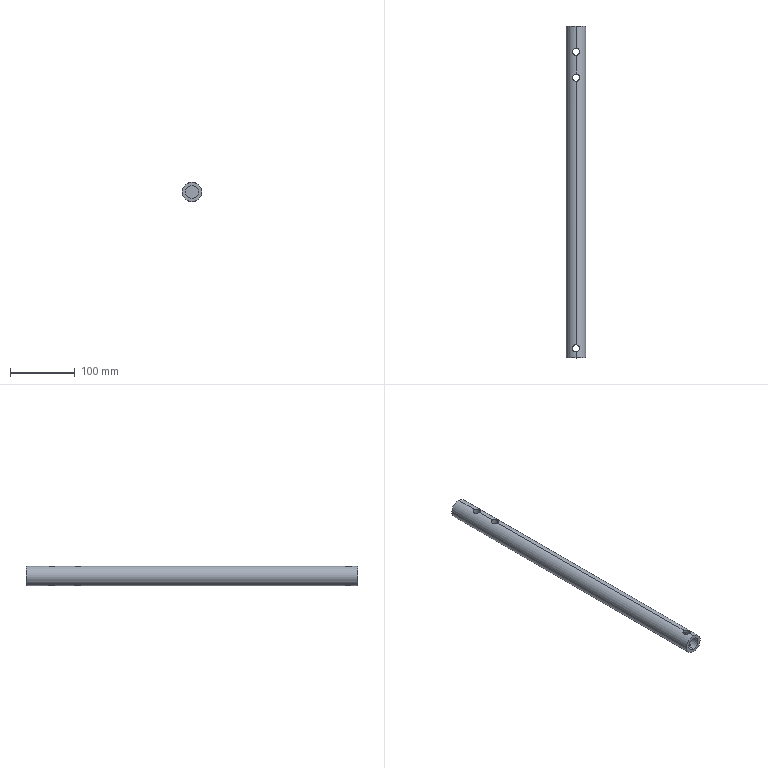Part | SolidWorks | features ICE 3, MoveFace 3, Extrusion 1 | 1 solid | 15 faces | box 30 x 514 x 30 mm | volume 341036 mm3 | cylinder 12 | plane 3 | commonest cylinder face diameters 11 x8 20 x2 30 x2